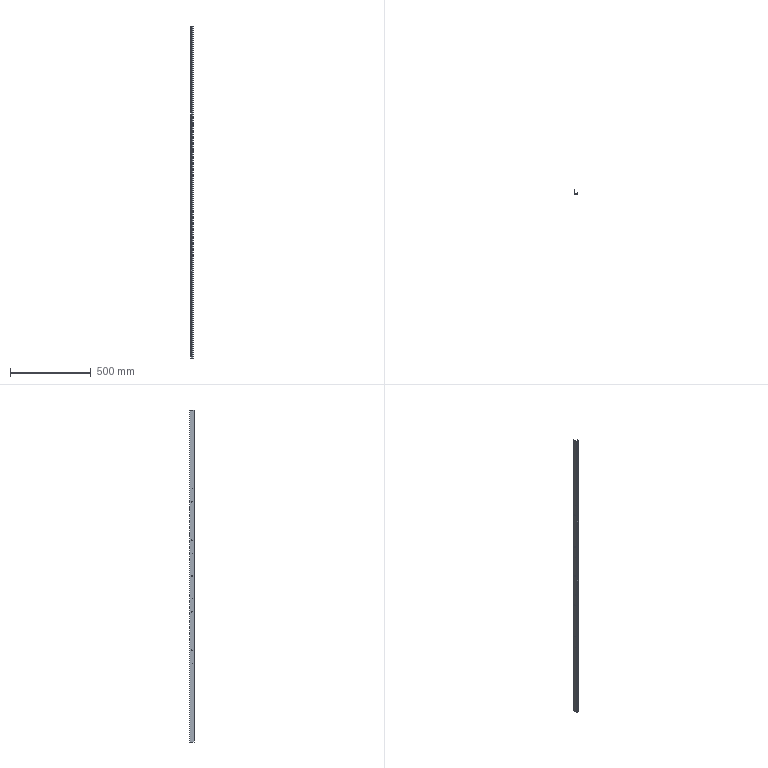Part | SolidWorks | features Cut 1, EdgeFlange 1, FlatPattern 1, ICE 1, SMBaseFlange 1, SheetMetal 1 | 1 solid | 72 faces | box 17 x 30 x 2056 mm | volume 161613 mm3 | plane 50 | cylinder 22 | commonest cylinder face diameters 6.1 x10 2 x6 5 x6